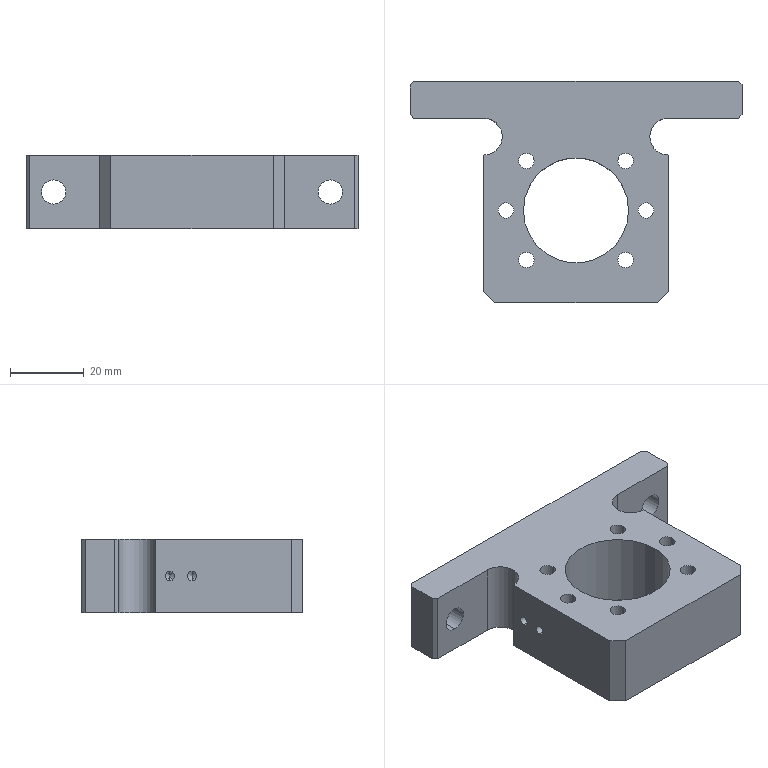Part | STEP file | 1 solid | 53 faces | box 90 x 60 x 20 mm | volume 50932 mm3 | cylinder 29 | plane 16 | cone 8 | commonest cylinder face diameters 4.2 x12 2.5 x8 6.6 x4 10 x3 28.5 x2